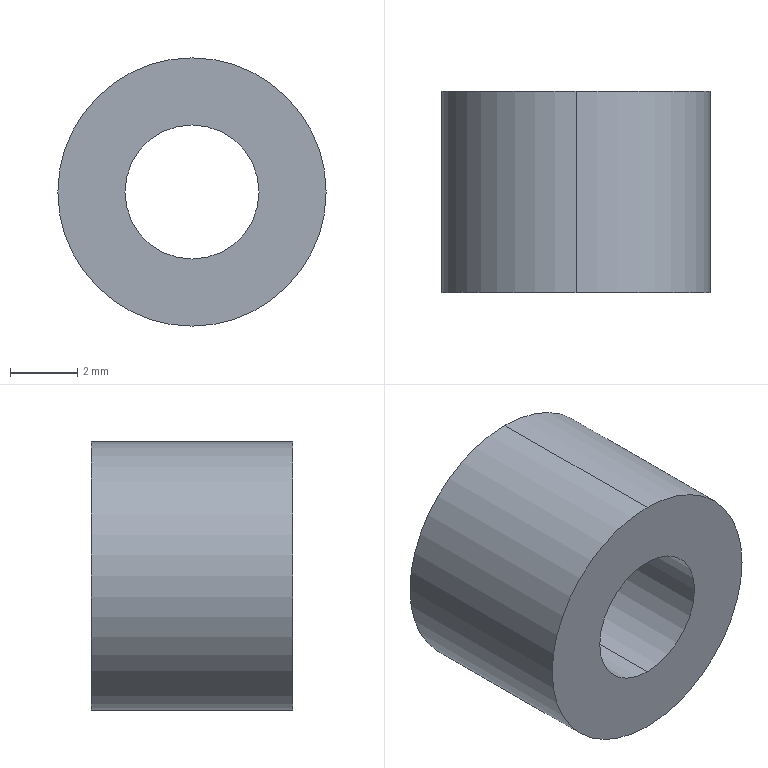Part | SolidWorks | features Revolution 1 | 1 solid | 6 faces | box 8 x 6 x 8 mm | volume 226.195 mm3 | cylinder 4 | plane 2 | commonest cylinder face diameters 4 x2 8 x2
STEP:
#1=CARTESIAN_POINT('',(0.,0.,4.));
#2=VERTEX_POINT('',#1);
#3=CARTESIAN_POINT('',(0.,0.,-4.));
#4=VERTEX_POINT('',#3);
#5=CARTESIAN_POINT('',(0.,0.,0.));
#6=DIRECTION('',(0.,1.,0.));
#7=DIRECTION('',(0.,0.,1.));
#8=AXIS2_PLACEMENT_3D('',#5,#6,#7);
#9=CIRCLE('',#8,4.);
#10=EDGE_CURVE('',#2,#4,#9,.T.);
#11=ORIENTED_EDGE('',*,*,#10,.T.);
#12=CARTESIAN_POINT('',(0.,6.,-4.));
#13=VERTEX_POINT('',#12);
#14=CARTESIAN_POINT('',(0.,8.416,-4.));
#15=DIRECTION('',(0.,1.,0.));
#16=VECTOR('',#15,1000.);
#17=LINE('',#14,#16);
#18=EDGE_CURVE('',#4,#13,#17,.T.);
#19=ORIENTED_EDGE('',*,*,#18,.T.);
#20=CARTESIAN_POINT('',(0.,6.,4.));
#21=VERTEX_POINT('',#20);
#22=CARTESIAN_POINT('',(0.,6.,0.));
#23=DIRECTION('',(0.,1.,0.));
#24=DIRECTION('',(0.,0.,1.));
#25=AXIS2_PLACEMENT_3D('',#22,#23,#24);
#26=CIRCLE('',#25,4.);
#27=EDGE_CURVE('',#21,#13,#26,.T.);
#28=ORIENTED_EDGE('',*,*,#27,.F.);
#29=CARTESIAN_POINT('',(0.,8.416,4.));
#30=DIRECTION('',(0.,1.,0.));
#31=VECTOR('',#30,1000.);
#32=LINE('',#29,#31);
#33=EDGE_CURVE('',#2,#21,#32,.T.);
#34=ORIENTED_EDGE('',*,*,#33,.F.);
#35=EDGE_LOOP('',(#11,#19,#28,#34));
#36=FACE_OUTER_BOUND('',#35,.T.);
#37=CARTESIAN_POINT('',(0.,8.416,0.));
#38=DIRECTION('',(0.,1.,0.));
#39=DIRECTION('',(0.,0.,1.));
#40=AXIS2_PLACEMENT_3D('',#37,#38,#39);
#41=CYLINDRICAL_SURFACE('',#40,4.);
#42=ADVANCED_FACE('',(#36),#41,.T.);
#43=CARTESIAN_POINT('',(0.,0.,-2.));
#44=VERTEX_POINT('',#43);
#45=CARTESIAN_POINT('',(0.,0.,2.));
#46=VERTEX_POINT('',#45);
#47=CARTESIAN_POINT('',(0.,0.,0.));
#48=DIRECTION('',(0.,1.,0.));
#49=DIRECTION('',(0.,0.,1.));
#50=AXIS2_PLACEMENT_3D('',#47,#48,#49);
#51=CIRCLE('',#50,2.);
#52=EDGE_CURVE('',#44,#46,#51,.T.);
#53=ORIENTED_EDGE('',*,*,#52,.F.);
#54=CARTESIAN_POINT('',(0.,6.,-2.));
#55=VERTEX_POINT('',#54);
#56=CARTESIAN_POINT('',(0.,8.416,-2.));
#57=DIRECTION('',(0.,1.,0.));
#58=VECTOR('',#57,1000.);
#59=LINE('',#56,#58);
#60=EDGE_CURVE('',#44,#55,#59,.T.);
#61=ORIENTED_EDGE('',*,*,#60,.T.);
#62=CARTESIAN_POINT('',(0.,6.,2.));
#63=VERTEX_POINT('',#62);
#64=CARTESIAN_POINT('',(0.,6.,0.));
#65=DIRECTION('',(0.,1.,0.));
#66=DIRECTION('',(0.,0.,1.));
#67=AXIS2_PLACEMENT_3D('',#64,#65,#66);
#68=CIRCLE('',#67,2.);
#69=EDGE_CURVE('',#55,#63,#68,.T.);
#70=ORIENTED_EDGE('',*,*,#69,.T.);
#71=CARTESIAN_POINT('',(0.,8.416,2.));
#72=DIRECTION('',(0.,1.,0.));
#73=VECTOR('',#72,1000.);
#74=LINE('',#71,#73);
#75=EDGE_CURVE('',#46,#63,#74,.T.);
#76=ORIENTED_EDGE('',*,*,#75,.F.);
#77=EDGE_LOOP('',(#53,#61,#70,#76));
#78=FACE_OUTER_BOUND('',#77,.T.);
#79=CARTESIAN_POINT('',(0.,8.416,0.));
#80=DIRECTION('',(0.,1.,0.));
#81=DIRECTION('',(0.,0.,1.));
#82=AXIS2_PLACEMENT_3D('',#79,#80,#81);
#83=CYLINDRICAL_SURFACE('',#82,2.);
#84=ADVANCED_FACE('',(#78),#83,.F.);
#85=ORIENTED_EDGE('',*,*,#60,.F.);
#86=CARTESIAN_POINT('',(0.,0.,0.));
#87=DIRECTION('',(0.,1.,0.));
#88=DIRECTION('',(0.,0.,1.));
#89=AXIS2_PLACEMENT_3D('',#86,#87,#88);
#90=CIRCLE('',#89,2.);
#91=EDGE_CURVE('',#46,#44,#90,.T.);
#92=ORIENTED_EDGE('',*,*,#91,.F.);
#93=ORIENTED_EDGE('',*,*,#75,.T.);
#94=CARTESIAN_POINT('',(0.,6.,0.));
#95=DIRECTION('',(0.,1.,0.));
#96=DIRECTION('',(0.,0.,1.));
#97=AXIS2_PLACEMENT_3D('',#94,#95,#96);
#98=CIRCLE('',#97,2.);
#99=EDGE_CURVE('',#63,#55,#98,.T.);
#100=ORIENTED_EDGE('',*,*,#99,.T.);
#101=EDGE_LOOP('',(#85,#92,#93,#100));
#102=FACE_OUTER_BOUND('',#101,.T.);
#103=CARTESIAN_POINT('',(0.,8.416,0.));
#104=DIRECTION('',(0.,1.,0.));
#105=DIRECTION('',(0.,0.,1.));
#106=AXIS2_PLACEMENT_3D('',#103,#104,#105);
#107=CYLINDRICAL_SURFACE('',#106,2.);
#108=ADVANCED_FACE('',(#102),#107,.F.);
#109=ORIENTED_EDGE('',*,*,#27,.T.);
#110=CARTESIAN_POINT('',(0.,6.,0.));
#111=DIRECTION('',(0.,1.,0.));
#112=DIRECTION('',(0.,0.,1.));
#113=AXIS2_PLACEMENT_3D('',#110,#111,#112);
#114=CIRCLE('',#113,4.);
#115=EDGE_CURVE('',#13,#21,#114,.T.);
#116=ORIENTED_EDGE('',*,*,#115,.T.);
#117=EDGE_LOOP('',(#109,#116));
#118=FACE_OUTER_BOUND('',#117,.T.);
#119=ORIENTED_EDGE('',*,*,#99,.F.);
#120=ORIENTED_EDGE('',*,*,#69,.F.);
#121=EDGE_LOOP('',(#119,#120));
#122=FACE_BOUND('',#121,.T.);
#123=CARTESIAN_POINT('',(-2.,6.,0.));
#124=DIRECTION('',(0.,1.,0.));
#125=DIRECTION('',(0.,0.,1.));
#126=AXIS2_PLACEMENT_3D('',#123,#124,#125);
#127=PLANE('',#126);
#128=ADVANCED_FACE('',(#118,#122),#127,.T.);
#129=ORIENTED_EDGE('',*,*,#18,.F.);
#130=CARTESIAN_POINT('',(0.,0.,0.));
#131=DIRECTION('',(0.,1.,0.));
#132=DIRECTION('',(0.,0.,1.));
#133=AXIS2_PLACEMENT_3D('',#130,#131,#132);
#134=CIRCLE('',#133,4.);
#135=EDGE_CURVE('',#4,#2,#134,.T.);
#136=ORIENTED_EDGE('',*,*,#135,.T.);
#137=ORIENTED_EDGE('',*,*,#33,.T.);
#138=ORIENTED_EDGE('',*,*,#115,.F.);
#139=EDGE_LOOP('',(#129,#136,#137,#138));
#140=FACE_OUTER_BOUND('',#139,.T.);
#141=CARTESIAN_POINT('',(0.,8.416,0.));
#142=DIRECTION('',(0.,1.,0.));
#143=DIRECTION('',(0.,0.,1.));
#144=AXIS2_PLACEMENT_3D('',#141,#142,#143);
#145=CYLINDRICAL_SURFACE('',#144,4.);
#146=ADVANCED_FACE('',(#140),#145,.T.);
#147=ORIENTED_EDGE('',*,*,#91,.T.);
#148=ORIENTED_EDGE('',*,*,#52,.T.);
#149=EDGE_LOOP('',(#147,#148));
#150=FACE_BOUND('',#149,.T.);
#151=ORIENTED_EDGE('',*,*,#10,.F.);
#152=ORIENTED_EDGE('',*,*,#135,.F.);
#153=EDGE_LOOP('',(#151,#152));
#154=FACE_OUTER_BOUND('',#153,.T.);
#155=CARTESIAN_POINT('',(-2.,0.,0.));
#156=DIRECTION('',(0.,-1.,0.));
#157=DIRECTION('',(0.,0.,-1.));
#158=AXIS2_PLACEMENT_3D('',#155,#156,#157);
#159=PLANE('',#158);
#160=ADVANCED_FACE('',(#150,#154),#159,.T.);
#161=CLOSED_SHELL('',(#42,#84,#108,#128,#146,#160));
#162=MANIFOLD_SOLID_BREP('',#161);
#163=CARTESIAN_POINT('',(0.,0.,0.));
#164=DIRECTION('',(0.,0.,1.));
#165=DIRECTION('',(1.,0.,0.));
#166=AXIS2_PLACEMENT_3D('',#163,#164,#165);
#167=(LENGTH_UNIT()NAMED_UNIT(*)SI_UNIT(.MILLI.,.METRE.));
#168=UNCERTAINTY_MEASURE_WITH_UNIT(LENGTH_MEASURE(0.00001),#167,'','');
#169=(NAMED_UNIT(*)PLANE_ANGLE_UNIT()SI_UNIT($,.RADIAN.));
#170=(NAMED_UNIT(*)SI_UNIT($,.STERADIAN.)SOLID_ANGLE_UNIT());
#171=(GEOMETRIC_REPRESENTATION_CONTEXT(3)GLOBAL_UNCERTAINTY_ASSIGNED_CONTEXT((#168))GLOBAL_UNIT_ASSIGNED_CONTEXT((#167,#169,#170))REPRESENTATION_CONTEXT('',''));
#172=ADVANCED_BREP_SHAPE_REPRESENTATION('',(#162,#166),#171);